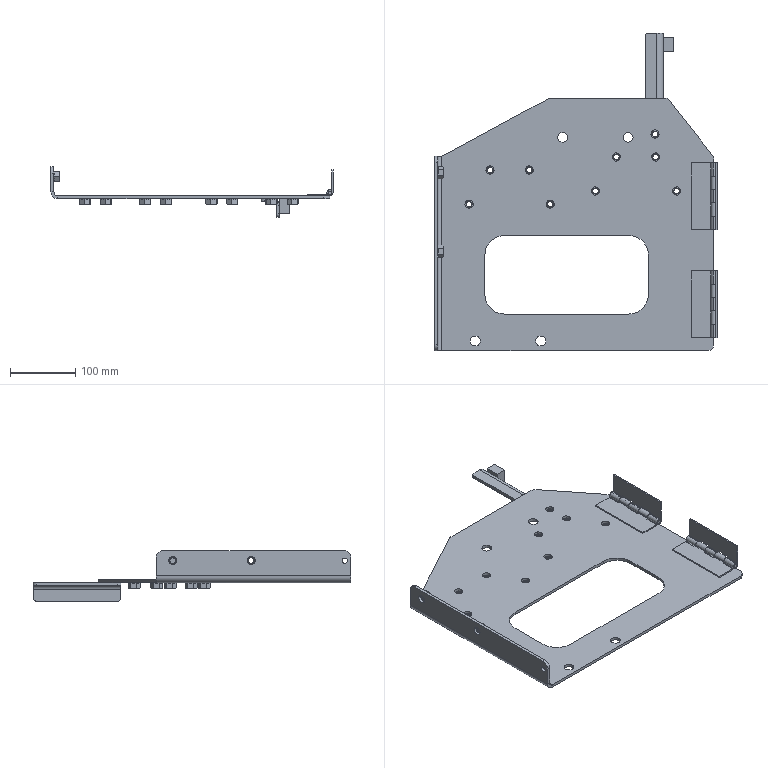Part | SolidWorks | features LocalLPattern 1, ReferencePattern 1 | 20 solids | 907 faces | box 430.7 x 485 x 77 mm | volume 689394 mm3 | cone 440 | cylinder 271 | plane 196 | commonest cylinder face diameters 8.376 x154 5.6 x34 9.4 x30 12.5 x22 15 x8 20 x7